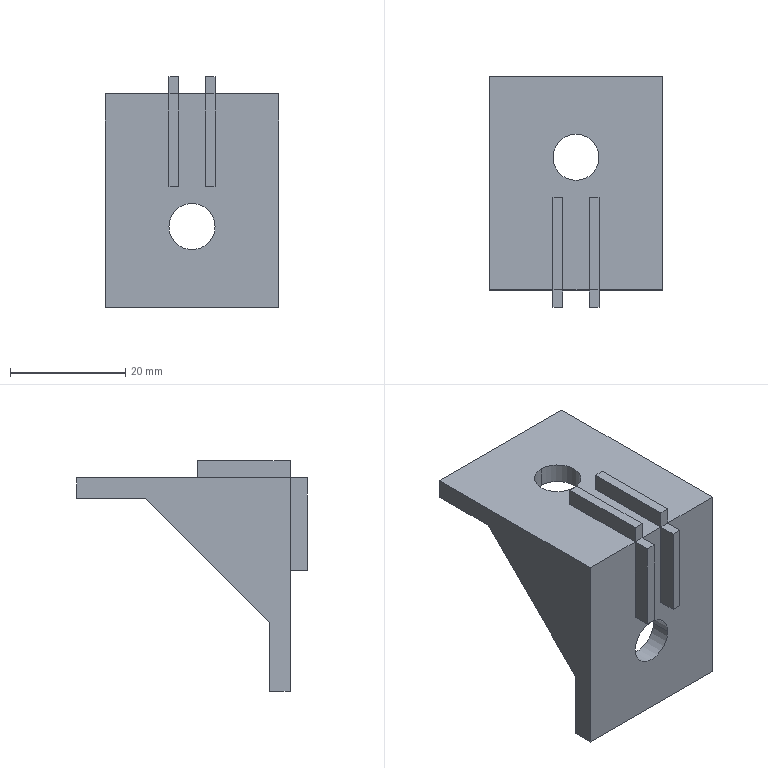Part | STEP file | 40×40 aluminium angle | 1 solid | 36 faces | box 30 x 40 x 40 mm | volume 8764 mm3 | plane 32 | cylinder 4 | commonest cylinder face diameters 8 x4